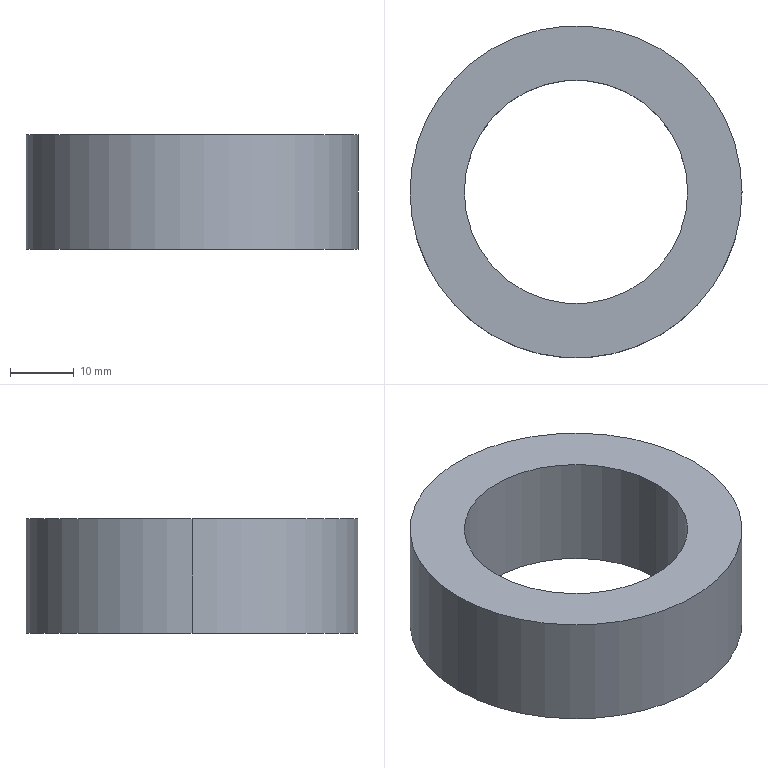Part | STEP file | Lock Nut | 1 solid | 6 faces | box 52 x 52 x 18 mm | volume 20909 mm3 | cylinder 4 | plane 2 | commonest cylinder face diameters 35 x2 52 x2
STEP:
#1=CARTESIAN_POINT('',(-26.,0.,18.));
#2=VERTEX_POINT('',#1);
#3=CARTESIAN_POINT('',(26.,0.,18.));
#4=VERTEX_POINT('',#3);
#5=CARTESIAN_POINT('',(0.,0.,18.));
#6=DIRECTION('',(0.,0.,-1.));
#7=DIRECTION('',(-1.,0.,0.));
#8=AXIS2_PLACEMENT_3D('',#5,#6,#7);
#9=CIRCLE('',#8,26.);
#10=EDGE_CURVE('',#2,#4,#9,.T.);
#11=ORIENTED_EDGE('',*,*,#10,.T.);
#12=CARTESIAN_POINT('',(26.,0.,0.));
#13=VERTEX_POINT('',#12);
#14=CARTESIAN_POINT('',(26.,0.,18.));
#15=DIRECTION('',(0.,0.,-1.));
#16=VECTOR('',#15,1000.);
#17=LINE('',#14,#16);
#18=EDGE_CURVE('',#4,#13,#17,.T.);
#19=ORIENTED_EDGE('',*,*,#18,.T.);
#20=CARTESIAN_POINT('',(-26.,0.,0.));
#21=VERTEX_POINT('',#20);
#22=CARTESIAN_POINT('',(0.,0.,0.));
#23=DIRECTION('',(0.,0.,1.));
#24=DIRECTION('',(-1.,0.,0.));
#25=AXIS2_PLACEMENT_3D('',#22,#23,#24);
#26=CIRCLE('',#25,26.);
#27=EDGE_CURVE('',#13,#21,#26,.T.);
#28=ORIENTED_EDGE('',*,*,#27,.T.);
#29=CARTESIAN_POINT('',(-26.,0.,18.));
#30=DIRECTION('',(0.,0.,-1.));
#31=VECTOR('',#30,1000.);
#32=LINE('',#29,#31);
#33=EDGE_CURVE('',#2,#21,#32,.T.);
#34=ORIENTED_EDGE('',*,*,#33,.F.);
#35=EDGE_LOOP('',(#11,#19,#28,#34));
#36=FACE_OUTER_BOUND('',#35,.T.);
#37=CARTESIAN_POINT('',(0.,0.,18.));
#38=DIRECTION('',(0.,0.,-1.));
#39=DIRECTION('',(-1.,0.,0.));
#40=AXIS2_PLACEMENT_3D('',#37,#38,#39);
#41=CYLINDRICAL_SURFACE('',#40,26.);
#42=ADVANCED_FACE('',(#36),#41,.T.);
#43=CARTESIAN_POINT('',(17.5,0.,18.));
#44=VERTEX_POINT('',#43);
#45=CARTESIAN_POINT('',(-17.5,0.,18.));
#46=VERTEX_POINT('',#45);
#47=CARTESIAN_POINT('',(0.,0.,18.));
#48=DIRECTION('',(0.,0.,-1.));
#49=DIRECTION('',(-1.,0.,0.));
#50=AXIS2_PLACEMENT_3D('',#47,#48,#49);
#51=CIRCLE('',#50,17.5);
#52=EDGE_CURVE('',#44,#46,#51,.T.);
#53=ORIENTED_EDGE('',*,*,#52,.F.);
#54=CARTESIAN_POINT('',(17.5,0.,0.));
#55=VERTEX_POINT('',#54);
#56=CARTESIAN_POINT('',(17.5,0.,18.));
#57=DIRECTION('',(0.,0.,-1.));
#58=VECTOR('',#57,1000.);
#59=LINE('',#56,#58);
#60=EDGE_CURVE('',#44,#55,#59,.T.);
#61=ORIENTED_EDGE('',*,*,#60,.T.);
#62=CARTESIAN_POINT('',(-17.5,0.,0.));
#63=VERTEX_POINT('',#62);
#64=CARTESIAN_POINT('',(0.,0.,0.));
#65=DIRECTION('',(0.,0.,-1.));
#66=DIRECTION('',(-1.,0.,0.));
#67=AXIS2_PLACEMENT_3D('',#64,#65,#66);
#68=CIRCLE('',#67,17.5);
#69=EDGE_CURVE('',#55,#63,#68,.T.);
#70=ORIENTED_EDGE('',*,*,#69,.T.);
#71=CARTESIAN_POINT('',(-17.5,0.,18.));
#72=DIRECTION('',(0.,0.,-1.));
#73=VECTOR('',#72,1000.);
#74=LINE('',#71,#73);
#75=EDGE_CURVE('',#46,#63,#74,.T.);
#76=ORIENTED_EDGE('',*,*,#75,.F.);
#77=EDGE_LOOP('',(#53,#61,#70,#76));
#78=FACE_OUTER_BOUND('',#77,.T.);
#79=CARTESIAN_POINT('',(0.,0.,18.));
#80=DIRECTION('',(0.,0.,-1.));
#81=DIRECTION('',(-1.,0.,0.));
#82=AXIS2_PLACEMENT_3D('',#79,#80,#81);
#83=CYLINDRICAL_SURFACE('',#82,17.5);
#84=ADVANCED_FACE('',(#78),#83,.F.);
#85=ORIENTED_EDGE('',*,*,#18,.F.);
#86=CARTESIAN_POINT('',(0.,0.,18.));
#87=DIRECTION('',(0.,0.,-1.));
#88=DIRECTION('',(-1.,0.,0.));
#89=AXIS2_PLACEMENT_3D('',#86,#87,#88);
#90=CIRCLE('',#89,26.);
#91=EDGE_CURVE('',#4,#2,#90,.T.);
#92=ORIENTED_EDGE('',*,*,#91,.T.);
#93=ORIENTED_EDGE('',*,*,#33,.T.);
#94=CARTESIAN_POINT('',(0.,0.,0.));
#95=DIRECTION('',(0.,0.,1.));
#96=DIRECTION('',(-1.,0.,0.));
#97=AXIS2_PLACEMENT_3D('',#94,#95,#96);
#98=CIRCLE('',#97,26.);
#99=EDGE_CURVE('',#21,#13,#98,.T.);
#100=ORIENTED_EDGE('',*,*,#99,.T.);
#101=EDGE_LOOP('',(#85,#92,#93,#100));
#102=FACE_OUTER_BOUND('',#101,.T.);
#103=CARTESIAN_POINT('',(0.,0.,18.));
#104=DIRECTION('',(0.,0.,-1.));
#105=DIRECTION('',(-1.,0.,0.));
#106=AXIS2_PLACEMENT_3D('',#103,#104,#105);
#107=CYLINDRICAL_SURFACE('',#106,26.);
#108=ADVANCED_FACE('',(#102),#107,.T.);
#109=CARTESIAN_POINT('',(0.,0.,0.));
#110=DIRECTION('',(0.,0.,-1.));
#111=DIRECTION('',(-1.,0.,0.));
#112=AXIS2_PLACEMENT_3D('',#109,#110,#111);
#113=CIRCLE('',#112,17.5);
#114=EDGE_CURVE('',#63,#55,#113,.T.);
#115=ORIENTED_EDGE('',*,*,#114,.F.);
#116=ORIENTED_EDGE('',*,*,#69,.F.);
#117=EDGE_LOOP('',(#115,#116));
#118=FACE_BOUND('',#117,.T.);
#119=ORIENTED_EDGE('',*,*,#99,.F.);
#120=ORIENTED_EDGE('',*,*,#27,.F.);
#121=EDGE_LOOP('',(#119,#120));
#122=FACE_OUTER_BOUND('',#121,.T.);
#123=CARTESIAN_POINT('',(0.,0.,0.));
#124=DIRECTION('',(0.,0.,1.));
#125=DIRECTION('',(1.,0.,0.));
#126=AXIS2_PLACEMENT_3D('',#123,#124,#125);
#127=PLANE('',#126);
#128=ADVANCED_FACE('',(#118,#122),#127,.F.);
#129=CARTESIAN_POINT('',(0.,0.,18.));
#130=DIRECTION('',(0.,0.,-1.));
#131=DIRECTION('',(-1.,0.,0.));
#132=AXIS2_PLACEMENT_3D('',#129,#130,#131);
#133=CIRCLE('',#132,17.5);
#134=EDGE_CURVE('',#46,#44,#133,.T.);
#135=ORIENTED_EDGE('',*,*,#134,.T.);
#136=ORIENTED_EDGE('',*,*,#52,.T.);
#137=EDGE_LOOP('',(#135,#136));
#138=FACE_BOUND('',#137,.T.);
#139=ORIENTED_EDGE('',*,*,#10,.F.);
#140=ORIENTED_EDGE('',*,*,#91,.F.);
#141=EDGE_LOOP('',(#139,#140));
#142=FACE_OUTER_BOUND('',#141,.T.);
#143=CARTESIAN_POINT('',(0.,0.,18.));
#144=DIRECTION('',(0.,0.,1.));
#145=DIRECTION('',(1.,0.,0.));
#146=AXIS2_PLACEMENT_3D('',#143,#144,#145);
#147=PLANE('',#146);
#148=ADVANCED_FACE('',(#138,#142),#147,.T.);
#149=ORIENTED_EDGE('',*,*,#60,.F.);
#150=ORIENTED_EDGE('',*,*,#134,.F.);
#151=ORIENTED_EDGE('',*,*,#75,.T.);
#152=ORIENTED_EDGE('',*,*,#114,.T.);
#153=EDGE_LOOP('',(#149,#150,#151,#152));
#154=FACE_OUTER_BOUND('',#153,.T.);
#155=CARTESIAN_POINT('',(0.,0.,18.));
#156=DIRECTION('',(0.,0.,-1.));
#157=DIRECTION('',(-1.,0.,0.));
#158=AXIS2_PLACEMENT_3D('',#155,#156,#157);
#159=CYLINDRICAL_SURFACE('',#158,17.5);
#160=ADVANCED_FACE('',(#154),#159,.F.);
#161=CLOSED_SHELL('',(#42,#84,#108,#128,#148,#160));
#162=MANIFOLD_SOLID_BREP('',#161);
#163=CARTESIAN_POINT('',(0.,0.,0.));
#164=DIRECTION('',(0.,0.,1.));
#165=DIRECTION('',(1.,0.,0.));
#166=AXIS2_PLACEMENT_3D('',#163,#164,#165);
#167=(LENGTH_UNIT()NAMED_UNIT(*)SI_UNIT(.MILLI.,.METRE.));
#168=UNCERTAINTY_MEASURE_WITH_UNIT(LENGTH_MEASURE(0.00001),#167,'','');
#169=(NAMED_UNIT(*)PLANE_ANGLE_UNIT()SI_UNIT($,.RADIAN.));
#170=(NAMED_UNIT(*)SI_UNIT($,.STERADIAN.)SOLID_ANGLE_UNIT());
#171=(GEOMETRIC_REPRESENTATION_CONTEXT(3)GLOBAL_UNCERTAINTY_ASSIGNED_CONTEXT((#168))GLOBAL_UNIT_ASSIGNED_CONTEXT((#167,#169,#170))REPRESENTATION_CONTEXT('',''));
#172=ADVANCED_BREP_SHAPE_REPRESENTATION('',(#162,#166),#171);